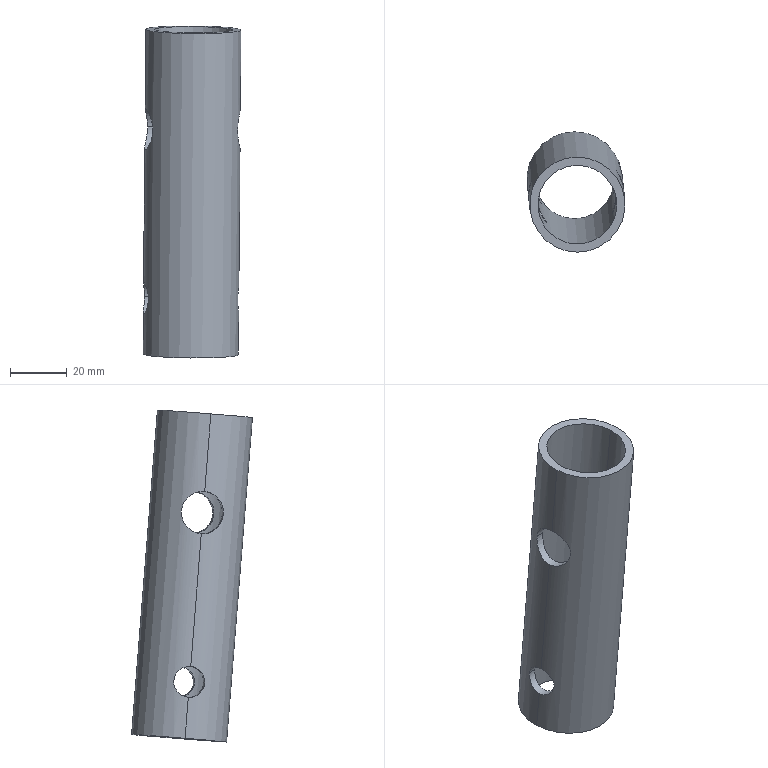Part | SolidWorks | features BaseBody 1 | 1 solid | 14 faces | box 34.667 x 42.72 x 117.323 mm | volume 30652 mm3 | cylinder 12 | plane 2 | commonest cylinder face diameters 11 x4 15 x4 27.9 x2 33.7 x2